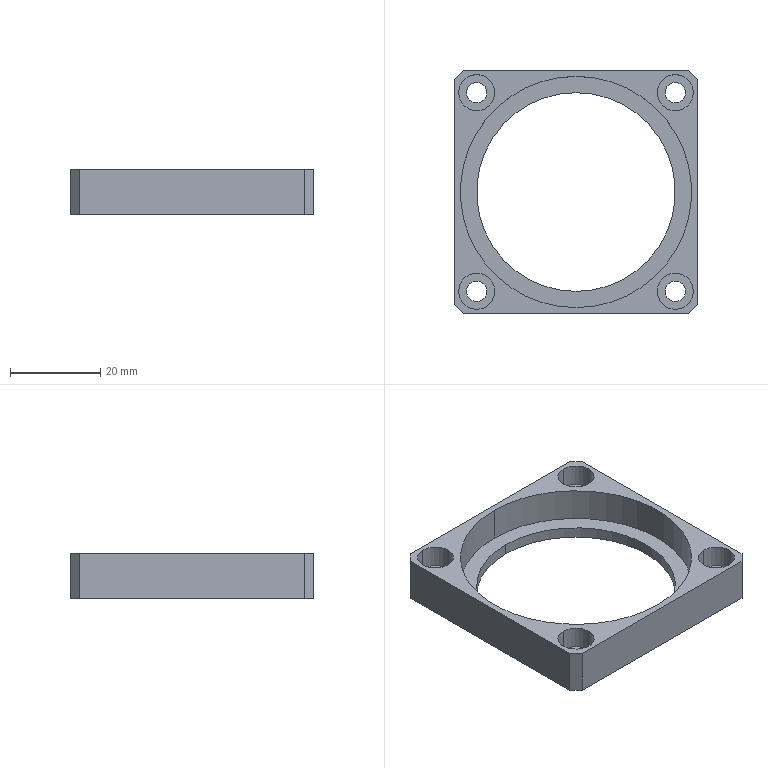CAM job | NX | 3-axis milling, drilling | part box 54 x 54 x 10 mm | stock box 58 x 58 x 10 mm
Tools:
number,name,description,diameter,corner_radius,flute_length,length,flutes
7,D6A45,Milling Tool-5 Parameters,6.0,0.0,50.0,75.0,2
14,4.5ZT,Drilling Tool,4.5,0.0,35.0,50.0,2
6,D6,Milling Tool-5 Parameters,6.0,0.0,50.0,75.0,2
10,D10,Milling Tool-5 Parameters,10.0,0.0,50.0,75.0,2
11,D10JING,Milling Tool-5 Parameters,10.0,0.0,50.0,75.0,2
Operations:
program,operation,operation_type,tool,method,geometry_group,spindle_rpm,surface_speed,feed_per_tooth,feed_cut,feed_plunge,cut_length_mm,path_length_mm,cut_time_min,machine_time_min
1,DRILLING,Operation,D6A45,METHOD,A,5000.0,94.0,0.025,250.0,0.0,20.0,262.718,0.08,0.1043
1,DRILLING_COPY,Operation,4.5ZT,METHOD,A,2000.0,28.0,0.0625,250.0,0.0,79.26,381.238,0.317,0.3472
1,HOLE_MILLING,CylinderMilling,D6,METHOD,A,9500.0,179.0,0.0789,1500.0,100.0,320.076,709.676,0.2134,0.2523
1,HOLE_MILLING_COPY,CylinderMilling,D10,METHOD,A,9500.0,298.0,0.1158,2200.0,100.0,5699.766,5790.966,2.591,2.6
1,HOLE_MILLING_COPY_COPY,CylinderMilling,D10,METHOD,A,9500.0,298.0,0.1158,2200.0,100.0,1635.302,1718.402,0.7433,0.7516
1,ZLEVEL_PROFILE,ZLevelMilling,D10,METHOD,A,9500.0,298.0,0.1316,2500.0,1000.0,4934.836,5001.686,1.997,2.003
1,ZLEVEL_PROFILE_COPY_COPY,ZLevelMilling,D10JING,METHOD,A,9500.0,298.0,0.0632,1200.0,1000.0,139.19,210.19,0.1168,0.1239
1,ZLEVEL_PROFILE_COPY_COPY_COPY,ZLevelMilling,D10JING,METHOD,A,9500.0,298.0,0.0632,1200.0,1000.0,116.621,192.621,0.098,0.1056
1,PLANAR_MILL,PlanarMilling,D6A45,METHOD,A,9500.0,179.0,0.0658,1250.0,100.0,480.641,1007.68,0.3845,0.4372
1,PLANAR_MILL_COPY,PlanarMilling,D6A45,METHOD,A,9500.0,179.0,0.0658,1250.0,100.0,137.67,211.67,0.1101,0.1175
1,ZLEVEL_PROFILE_COPY,ZLevelMilling,D10JING,METHOD,A,9500.0,298.0,0.0632,1200.0,1000.0,991.423,1058.323,0.8469,0.8536